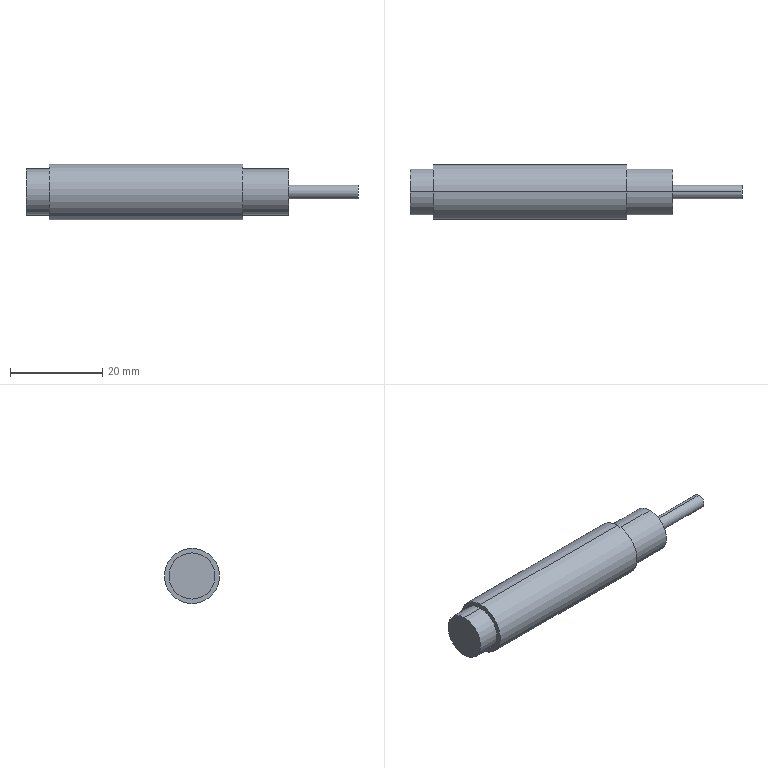Part | STEP file | PN_0014_default | 1 solid | 13 faces | box 72 x 12 x 12 mm | volume 6034 mm3 | cylinder 8 | plane 5 | commonest cylinder face diameters 10 x4 3 x2 12 x2
STEP:
#1=CARTESIAN_POINT('',(0.,0.,0.));
#2=DIRECTION('',(0.,0.,1.));
#3=DIRECTION('',(1.,0.,0.));
#4=AXIS2_PLACEMENT_3D('',#1,#2,#3);
#5=CARTESIAN_POINT('',(72.,0.,-1.5));
#6=VERTEX_POINT('',#5);
#7=CARTESIAN_POINT('',(72.,0.,1.5));
#8=VERTEX_POINT('',#7);
#9=CARTESIAN_POINT('',(72.,0.,0.));
#10=DIRECTION('',(1.,0.,0.));
#11=DIRECTION('',(0.,0.,-1.));
#12=AXIS2_PLACEMENT_3D('',#9,#10,#11);
#13=CIRCLE('',#12,1.5);
#14=CARTESIAN_POINT('',(72.,0.,0.));
#15=DIRECTION('',(-1.,0.,0.));
#16=DIRECTION('',(0.,0.,1.));
#17=AXIS2_PLACEMENT_3D('',#14,#15,#16);
#18=CYLINDRICAL_SURFACE('',#17,1.5);
#19=CARTESIAN_POINT('',(3.142,0.));
#20=DIRECTION('',(-1.,0.));
#21=VECTOR('',#20,1.);
#22=LINE('',#19,#21);
#23=(GEOMETRIC_REPRESENTATION_CONTEXT(2)PARAMETRIC_REPRESENTATION_CONTEXT()REPRESENTATION_CONTEXT('',''));
#24=DEFINITIONAL_REPRESENTATION('',(#22),#23);
#25=PCURVE('',#18,#24);
#26=CARTESIAN_POINT('',(72.,0.,0.));
#27=DIRECTION('',(1.,0.,0.));
#28=DIRECTION('',(0.,0.,-1.));
#29=AXIS2_PLACEMENT_3D('',#26,#27,#28);
#30=PLANE('',#29);
#31=CARTESIAN_POINT('',(0.,0.));
#32=DIRECTION('',(1.,0.));
#33=AXIS2_PLACEMENT_2D('',#31,#32);
#34=CIRCLE('',#33,1.5);
#35=(GEOMETRIC_REPRESENTATION_CONTEXT(2)PARAMETRIC_REPRESENTATION_CONTEXT()REPRESENTATION_CONTEXT('',''));
#36=DEFINITIONAL_REPRESENTATION('',(#34),#35);
#37=PCURVE('',#30,#36);
#38=SURFACE_CURVE('',#13,(#25,#37),.PCURVE_S1.);
#39=EDGE_CURVE('',#6,#8,#38,.T.);
#40=ORIENTED_EDGE('',*,*,#39,.F.);
#41=CARTESIAN_POINT('',(57.,0.,-1.5));
#42=VERTEX_POINT('',#41);
#43=CARTESIAN_POINT('',(72.,0.,-1.5));
#44=DIRECTION('',(-1.,0.,0.));
#45=VECTOR('',#44,1.);
#46=LINE('',#43,#45);
#47=CARTESIAN_POINT('',(3.142,0.));
#48=DIRECTION('',(0.,1.));
#49=VECTOR('',#48,1.);
#50=LINE('',#47,#49);
#51=(GEOMETRIC_REPRESENTATION_CONTEXT(2)PARAMETRIC_REPRESENTATION_CONTEXT()REPRESENTATION_CONTEXT('',''));
#52=DEFINITIONAL_REPRESENTATION('',(#50),#51);
#53=PCURVE('',#18,#52);
#54=CARTESIAN_POINT('',(72.,0.,0.));
#55=DIRECTION('',(-1.,0.,0.));
#56=DIRECTION('',(0.,0.,1.));
#57=AXIS2_PLACEMENT_3D('',#54,#55,#56);
#58=CYLINDRICAL_SURFACE('',#57,1.5);
#59=CARTESIAN_POINT('',(3.142,0.));
#60=DIRECTION('',(0.,1.));
#61=VECTOR('',#60,1.);
#62=LINE('',#59,#61);
#63=(GEOMETRIC_REPRESENTATION_CONTEXT(2)PARAMETRIC_REPRESENTATION_CONTEXT()REPRESENTATION_CONTEXT('',''));
#64=DEFINITIONAL_REPRESENTATION('',(#62),#63);
#65=PCURVE('',#58,#64);
#66=SURFACE_CURVE('',#46,(#53,#65),.PCURVE_S1.);
#67=EDGE_CURVE('',#6,#42,#66,.T.);
#68=ORIENTED_EDGE('',*,*,#67,.T.);
#69=CARTESIAN_POINT('',(57.,0.,1.5));
#70=VERTEX_POINT('',#69);
#71=CARTESIAN_POINT('',(57.,0.,0.));
#72=DIRECTION('',(1.,0.,0.));
#73=DIRECTION('',(0.,0.,1.));
#74=AXIS2_PLACEMENT_3D('',#71,#72,#73);
#75=CIRCLE('',#74,1.5);
#76=CARTESIAN_POINT('',(6.283,15.));
#77=DIRECTION('',(-1.,0.));
#78=VECTOR('',#77,1.);
#79=LINE('',#76,#78);
#80=(GEOMETRIC_REPRESENTATION_CONTEXT(2)PARAMETRIC_REPRESENTATION_CONTEXT()REPRESENTATION_CONTEXT('',''));
#81=DEFINITIONAL_REPRESENTATION('',(#79),#80);
#82=PCURVE('',#18,#81);
#83=CARTESIAN_POINT('',(57.,5.,0.));
#84=DIRECTION('',(-1.,0.,0.));
#85=DIRECTION('',(0.,0.,1.));
#86=AXIS2_PLACEMENT_3D('',#83,#84,#85);
#87=PLANE('',#86);
#88=CARTESIAN_POINT('',(1.5,-5.));
#89=CARTESIAN_POINT('',(1.5,-7.598));
#90=CARTESIAN_POINT('',(-0.75,-6.299));
#91=CARTESIAN_POINT('',(-3.,-5.));
#92=CARTESIAN_POINT('',(-0.75,-3.701));
#93=CARTESIAN_POINT('',(1.5,-2.402));
#94=CARTESIAN_POINT('',(1.5,-5.));
#95=(BOUNDED_CURVE()B_SPLINE_CURVE(2,(#88,#89,#90,#91,#92,#93,#94),.UNSPECIFIED.,.T.,.F.)B_SPLINE_CURVE_WITH_KNOTS((1,2,2,2,2,1),(-2.094,0.,2.094,4.189,6.283,8.378),.UNSPECIFIED.)CURVE()GEOMETRIC_REPRESENTATION_ITEM()RATIONAL_B_SPLINE_CURVE((1.,0.5,1.,0.5,1.,0.5,1.))REPRESENTATION_ITEM(''));
#96=(GEOMETRIC_REPRESENTATION_CONTEXT(2)PARAMETRIC_REPRESENTATION_CONTEXT()REPRESENTATION_CONTEXT('',''));
#97=DEFINITIONAL_REPRESENTATION('',(#95),#96);
#98=PCURVE('',#87,#97);
#99=SURFACE_CURVE('',#75,(#82,#98),.PCURVE_S1.);
#100=EDGE_CURVE('',#42,#70,#99,.T.);
#101=ORIENTED_EDGE('',*,*,#100,.T.);
#102=CARTESIAN_POINT('',(72.,0.,1.5));
#103=DIRECTION('',(-1.,0.,0.));
#104=VECTOR('',#103,1.);
#105=LINE('',#102,#104);
#106=CARTESIAN_POINT('',(0.,0.));
#107=DIRECTION('',(0.,1.));
#108=VECTOR('',#107,1.);
#109=LINE('',#106,#108);
#110=(GEOMETRIC_REPRESENTATION_CONTEXT(2)PARAMETRIC_REPRESENTATION_CONTEXT()REPRESENTATION_CONTEXT('',''));
#111=DEFINITIONAL_REPRESENTATION('',(#109),#110);
#112=PCURVE('',#18,#111);
#113=CARTESIAN_POINT('',(6.283,0.));
#114=DIRECTION('',(0.,1.));
#115=VECTOR('',#114,1.);
#116=LINE('',#113,#115);
#117=(GEOMETRIC_REPRESENTATION_CONTEXT(2)PARAMETRIC_REPRESENTATION_CONTEXT()REPRESENTATION_CONTEXT('',''));
#118=DEFINITIONAL_REPRESENTATION('',(#116),#117);
#119=PCURVE('',#58,#118);
#120=SURFACE_CURVE('',#105,(#112,#119),.PCURVE_S1.);
#121=EDGE_CURVE('',#8,#70,#120,.T.);
#122=ORIENTED_EDGE('',*,*,#121,.F.);
#123=EDGE_LOOP('',(#40,#68,#101,#122));
#124=FACE_BOUND('',#123,.T.);
#125=ADVANCED_FACE('',(#124),#18,.T.);
#126=CARTESIAN_POINT('',(57.,0.,5.));
#127=VERTEX_POINT('',#126);
#128=CARTESIAN_POINT('',(57.,0.,-5.));
#129=VERTEX_POINT('',#128);
#130=CARTESIAN_POINT('',(57.,0.,0.));
#131=DIRECTION('',(-1.,0.,0.));
#132=DIRECTION('',(0.,0.,1.));
#133=AXIS2_PLACEMENT_3D('',#130,#131,#132);
#134=CIRCLE('',#133,5.);
#135=CARTESIAN_POINT('',(0.,0.,0.));
#136=DIRECTION('',(-1.,0.,0.));
#137=DIRECTION('',(0.,0.,1.));
#138=AXIS2_PLACEMENT_3D('',#135,#136,#137);
#139=CYLINDRICAL_SURFACE('',#138,5.);
#140=CARTESIAN_POINT('',(0.,-57.));
#141=DIRECTION('',(1.,0.));
#142=VECTOR('',#141,1.);
#143=LINE('',#140,#142);
#144=(GEOMETRIC_REPRESENTATION_CONTEXT(2)PARAMETRIC_REPRESENTATION_CONTEXT()REPRESENTATION_CONTEXT('',''));
#145=DEFINITIONAL_REPRESENTATION('',(#143),#144);
#146=PCURVE('',#139,#145);
#147=CARTESIAN_POINT('',(0.,-5.));
#148=DIRECTION('',(1.,0.));
#149=AXIS2_PLACEMENT_2D('',#147,#148);
#150=CIRCLE('',#149,5.);
#151=(GEOMETRIC_REPRESENTATION_CONTEXT(2)PARAMETRIC_REPRESENTATION_CONTEXT()REPRESENTATION_CONTEXT('',''));
#152=DEFINITIONAL_REPRESENTATION('',(#150),#151);
#153=PCURVE('',#87,#152);
#154=SURFACE_CURVE('',#134,(#146,#153),.PCURVE_S1.);
#155=EDGE_CURVE('',#127,#129,#154,.T.);
#156=ORIENTED_EDGE('',*,*,#155,.T.);
#157=CARTESIAN_POINT('',(47.,0.,-5.));
#158=VERTEX_POINT('',#157);
#159=CARTESIAN_POINT('',(0.,0.,-5.));
#160=DIRECTION('',(-1.,0.,0.));
#161=VECTOR('',#160,1.);
#162=LINE('',#159,#161);
#163=CARTESIAN_POINT('',(3.142,0.));
#164=DIRECTION('',(0.,1.));
#165=VECTOR('',#164,1.);
#166=LINE('',#163,#165);
#167=(GEOMETRIC_REPRESENTATION_CONTEXT(2)PARAMETRIC_REPRESENTATION_CONTEXT()REPRESENTATION_CONTEXT('',''));
#168=DEFINITIONAL_REPRESENTATION('',(#166),#167);
#169=PCURVE('',#139,#168);
#170=CARTESIAN_POINT('',(0.,0.,0.));
#171=DIRECTION('',(-1.,0.,0.));
#172=DIRECTION('',(0.,0.,1.));
#173=AXIS2_PLACEMENT_3D('',#170,#171,#172);
#174=CYLINDRICAL_SURFACE('',#173,5.);
#175=CARTESIAN_POINT('',(3.142,0.));
#176=DIRECTION('',(0.,1.));
#177=VECTOR('',#176,1.);
#178=LINE('',#175,#177);
#179=(GEOMETRIC_REPRESENTATION_CONTEXT(2)PARAMETRIC_REPRESENTATION_CONTEXT()REPRESENTATION_CONTEXT('',''));
#180=DEFINITIONAL_REPRESENTATION('',(#178),#179);
#181=PCURVE('',#174,#180);
#182=SURFACE_CURVE('',#162,(#169,#181),.PCURVE_S1.);
#183=EDGE_CURVE('',#129,#158,#182,.T.);
#184=ORIENTED_EDGE('',*,*,#183,.T.);
#185=CARTESIAN_POINT('',(47.,0.,5.));
#186=VERTEX_POINT('',#185);
#187=CARTESIAN_POINT('',(47.,0.,0.));
#188=DIRECTION('',(-1.,0.,0.));
#189=DIRECTION('',(0.,0.,1.));
#190=AXIS2_PLACEMENT_3D('',#187,#188,#189);
#191=CIRCLE('',#190,5.);
#192=CARTESIAN_POINT('',(0.,-47.));
#193=DIRECTION('',(1.,0.));
#194=VECTOR('',#193,1.);
#195=LINE('',#192,#194);
#196=(GEOMETRIC_REPRESENTATION_CONTEXT(2)PARAMETRIC_REPRESENTATION_CONTEXT()REPRESENTATION_CONTEXT('',''));
#197=DEFINITIONAL_REPRESENTATION('',(#195),#196);
#198=PCURVE('',#139,#197);
#199=CARTESIAN_POINT('',(47.,6.,0.));
#200=DIRECTION('',(-1.,0.,0.));
#201=DIRECTION('',(0.,0.,1.));
#202=AXIS2_PLACEMENT_3D('',#199,#200,#201);
#203=PLANE('',#202);
#204=CARTESIAN_POINT('',(0.,-6.));
#205=DIRECTION('',(1.,0.));
#206=AXIS2_PLACEMENT_2D('',#204,#205);
#207=CIRCLE('',#206,5.);
#208=(GEOMETRIC_REPRESENTATION_CONTEXT(2)PARAMETRIC_REPRESENTATION_CONTEXT()REPRESENTATION_CONTEXT('',''));
#209=DEFINITIONAL_REPRESENTATION('',(#207),#208);
#210=PCURVE('',#203,#209);
#211=SURFACE_CURVE('',#191,(#198,#210),.PCURVE_S1.);
#212=EDGE_CURVE('',#186,#158,#211,.T.);
#213=ORIENTED_EDGE('',*,*,#212,.F.);
#214=CARTESIAN_POINT('',(0.,0.,5.));
#215=DIRECTION('',(-1.,0.,0.));
#216=VECTOR('',#215,1.);
#217=LINE('',#214,#216);
#218=CARTESIAN_POINT('',(0.,0.));
#219=DIRECTION('',(0.,1.));
#220=VECTOR('',#219,1.);
#221=LINE('',#218,#220);
#222=(GEOMETRIC_REPRESENTATION_CONTEXT(2)PARAMETRIC_REPRESENTATION_CONTEXT()REPRESENTATION_CONTEXT('',''));
#223=DEFINITIONAL_REPRESENTATION('',(#221),#222);
#224=PCURVE('',#139,#223);
#225=CARTESIAN_POINT('',(6.283,0.));
#226=DIRECTION('',(0.,1.));
#227=VECTOR('',#226,1.);
#228=LINE('',#225,#227);
#229=(GEOMETRIC_REPRESENTATION_CONTEXT(2)PARAMETRIC_REPRESENTATION_CONTEXT()REPRESENTATION_CONTEXT('',''));
#230=DEFINITIONAL_REPRESENTATION('',(#228),#229);
#231=PCURVE('',#174,#230);
#232=SURFACE_CURVE('',#217,(#224,#231),.PCURVE_S1.);
#233=EDGE_CURVE('',#127,#186,#232,.T.);
#234=ORIENTED_EDGE('',*,*,#233,.F.);
#235=EDGE_LOOP('',(#156,#184,#213,#234));
#236=FACE_BOUND('',#235,.T.);
#237=ADVANCED_FACE('',(#236),#139,.T.);
#238=CARTESIAN_POINT('',(47.,0.,6.));
#239=VERTEX_POINT('',#238);
#240=CARTESIAN_POINT('',(47.,0.,-6.));
#241=VERTEX_POINT('',#240);
#242=CARTESIAN_POINT('',(47.,0.,0.));
#243=DIRECTION('',(-1.,0.,0.));
#244=DIRECTION('',(0.,0.,1.));
#245=AXIS2_PLACEMENT_3D('',#242,#243,#244);
#246=CIRCLE('',#245,6.);
#247=CARTESIAN_POINT('',(0.,0.,0.));
#248=DIRECTION('',(-1.,0.,0.));
#249=DIRECTION('',(0.,0.,1.));
#250=AXIS2_PLACEMENT_3D('',#247,#248,#249);
#251=CYLINDRICAL_SURFACE('',#250,6.);
#252=CARTESIAN_POINT('',(0.,-47.));
#253=DIRECTION('',(1.,0.));
#254=VECTOR('',#253,1.);
#255=LINE('',#252,#254);
#256=(GEOMETRIC_REPRESENTATION_CONTEXT(2)PARAMETRIC_REPRESENTATION_CONTEXT()REPRESENTATION_CONTEXT('',''));
#257=DEFINITIONAL_REPRESENTATION('',(#255),#256);
#258=PCURVE('',#251,#257);
#259=CARTESIAN_POINT('',(0.,-6.));
#260=DIRECTION('',(1.,0.));
#261=AXIS2_PLACEMENT_2D('',#259,#260);
#262=CIRCLE('',#261,6.);
#263=(GEOMETRIC_REPRESENTATION_CONTEXT(2)PARAMETRIC_REPRESENTATION_CONTEXT()REPRESENTATION_CONTEXT('',''));
#264=DEFINITIONAL_REPRESENTATION('',(#262),#263);
#265=PCURVE('',#203,#264);
#266=SURFACE_CURVE('',#246,(#258,#265),.PCURVE_S1.);
#267=EDGE_CURVE('',#239,#241,#266,.T.);
#268=ORIENTED_EDGE('',*,*,#267,.T.);
#269=CARTESIAN_POINT('',(5.,0.,-6.));
#270=VERTEX_POINT('',#269);
#271=CARTESIAN_POINT('',(0.,0.,-6.));
#272=DIRECTION('',(-1.,0.,0.));
#273=VECTOR('',#272,1.);
#274=LINE('',#271,#273);
#275=CARTESIAN_POINT('',(3.142,0.));
#276=DIRECTION('',(0.,1.));
#277=VECTOR('',#276,1.);
#278=LINE('',#275,#277);
#279=(GEOMETRIC_REPRESENTATION_CONTEXT(2)PARAMETRIC_REPRESENTATION_CONTEXT()REPRESENTATION_CONTEXT('',''));
#280=DEFINITIONAL_REPRESENTATION('',(#278),#279);
#281=PCURVE('',#251,#280);
#282=CARTESIAN_POINT('',(0.,0.,0.));
#283=DIRECTION('',(-1.,0.,0.));
#284=DIRECTION('',(0.,0.,1.));
#285=AXIS2_PLACEMENT_3D('',#282,#283,#284);
#286=CYLINDRICAL_SURFACE('',#285,6.);
#287=CARTESIAN_POINT('',(3.142,0.));
#288=DIRECTION('',(0.,1.));
#289=VECTOR('',#288,1.);
#290=LINE('',#287,#289);
#291=(GEOMETRIC_REPRESENTATION_CONTEXT(2)PARAMETRIC_REPRESENTATION_CONTEXT()REPRESENTATION_CONTEXT('',''));
#292=DEFINITIONAL_REPRESENTATION('',(#290),#291);
#293=PCURVE('',#286,#292);
#294=SURFACE_CURVE('',#274,(#281,#293),.PCURVE_S1.);
#295=EDGE_CURVE('',#241,#270,#294,.T.);
#296=ORIENTED_EDGE('',*,*,#295,.T.);
#297=CARTESIAN_POINT('',(5.,0.,6.));
#298=VERTEX_POINT('',#297);
#299=CARTESIAN_POINT('',(5.,0.,0.));
#300=DIRECTION('',(-1.,0.,0.));
#301=DIRECTION('',(0.,0.,1.));
#302=AXIS2_PLACEMENT_3D('',#299,#300,#301);
#303=CIRCLE('',#302,6.);
#304=CARTESIAN_POINT('',(0.,-5.));
#305=DIRECTION('',(1.,0.));
#306=VECTOR('',#305,1.);
#307=LINE('',#304,#306);
#308=(GEOMETRIC_REPRESENTATION_CONTEXT(2)PARAMETRIC_REPRESENTATION_CONTEXT()REPRESENTATION_CONTEXT('',''));
#309=DEFINITIONAL_REPRESENTATION('',(#307),#308);
#310=PCURVE('',#251,#309);
#311=CARTESIAN_POINT('',(5.,5.,0.));
#312=DIRECTION('',(1.,0.,0.));
#313=DIRECTION('',(0.,0.,-1.));
#314=AXIS2_PLACEMENT_3D('',#311,#312,#313);
#315=PLANE('',#314);
#316=CARTESIAN_POINT('',(-6.,-5.));
#317=CARTESIAN_POINT('',(-6.,5.392));
#318=CARTESIAN_POINT('',(3.,0.1962));
#319=CARTESIAN_POINT('',(12.,-5.));
#320=CARTESIAN_POINT('',(3.,-10.196));
#321=CARTESIAN_POINT('',(-6.,-15.392));
#322=CARTESIAN_POINT('',(-6.,-5.));
#323=(BOUNDED_CURVE()B_SPLINE_CURVE(2,(#316,#317,#318,#319,#320,#321,#322),.UNSPECIFIED.,.T.,.F.)B_SPLINE_CURVE_WITH_KNOTS((1,2,2,2,2,1),(-2.094,0.,2.094,4.189,6.283,8.378),.UNSPECIFIED.)CURVE()GEOMETRIC_REPRESENTATION_ITEM()RATIONAL_B_SPLINE_CURVE((1.,0.5,1.,0.5,1.,0.5,1.))REPRESENTATION_ITEM(''));
#324=(GEOMETRIC_REPRESENTATION_CONTEXT(2)PARAMETRIC_REPRESENTATION_CONTEXT()REPRESENTATION_CONTEXT('',''));
#325=DEFINITIONAL_REPRESENTATION('',(#323),#324);
#326=PCURVE('',#315,#325);
#327=SURFACE_CURVE('',#303,(#310,#326),.PCURVE_S1.);
#328=EDGE_CURVE('',#298,#270,#327,.T.);
#329=ORIENTED_EDGE('',*,*,#328,.F.);
#330=CARTESIAN_POINT('',(0.,0.,6.));
#331=DIRECTION('',(-1.,0.,0.));
#332=VECTOR('',#331,1.);
#333=LINE('',#330,#332);
#334=CARTESIAN_POINT('',(0.,0.));
#335=DIRECTION('',(0.,1.));
#336=VECTOR('',#335,1.);
#337=LINE('',#334,#336);
#338=(GEOMETRIC_REPRESENTATION_CONTEXT(2)PARAMETRIC_REPRESENTATION_CONTEXT()REPRESENTATION_CONTEXT('',''));
#339=DEFINITIONAL_REPRESENTATION('',(#337),#338);
#340=PCURVE('',#251,#339);
#341=CARTESIAN_POINT('',(6.283,0.));
#342=DIRECTION('',(0.,1.));
#343=VECTOR('',#342,1.);
#344=LINE('',#341,#343);
#345=(GEOMETRIC_REPRESENTATION_CONTEXT(2)PARAMETRIC_REPRESENTATION_CONTEXT()REPRESENTATION_CONTEXT('',''));
#346=DEFINITIONAL_REPRESENTATION('',(#344),#345);
#347=PCURVE('',#286,#346);
#348=SURFACE_CURVE('',#333,(#340,#347),.PCURVE_S1.);
#349=EDGE_CURVE('',#239,#298,#348,.T.);
#350=ORIENTED_EDGE('',*,*,#349,.F.);
#351=EDGE_LOOP('',(#268,#296,#329,#350));
#352=FACE_BOUND('',#351,.T.);
#353=ADVANCED_FACE('',(#352),#251,.T.);
#354=CARTESIAN_POINT('',(5.,0.,5.));
#355=VERTEX_POINT('',#354);
#356=CARTESIAN_POINT('',(5.,0.,-5.));
#357=VERTEX_POINT('',#356);
#358=CARTESIAN_POINT('',(5.,0.,0.));
#359=DIRECTION('',(-1.,0.,0.));
#360=DIRECTION('',(0.,0.,1.));
#361=AXIS2_PLACEMENT_3D('',#358,#359,#360);
#362=CIRCLE('',#361,5.);
#363=CARTESIAN_POINT('',(0.,0.,0.));
#364=DIRECTION('',(-1.,0.,0.));
#365=DIRECTION('',(0.,0.,1.));
#366=AXIS2_PLACEMENT_3D('',#363,#364,#365);
#367=CYLINDRICAL_SURFACE('',#366,5.);
#368=CARTESIAN_POINT('',(0.,-5.));
#369=DIRECTION('',(1.,0.));
#370=VECTOR('',#369,1.);
#371=LINE('',#368,#370);
#372=(GEOMETRIC_REPRESENTATION_CONTEXT(2)PARAMETRIC_REPRESENTATION_CONTEXT()REPRESENTATION_CONTEXT('',''));
#373=DEFINITIONAL_REPRESENTATION('',(#371),#372);
#374=PCURVE('',#367,#373);
#375=CARTESIAN_POINT('',(-5.,-5.));
#376=CARTESIAN_POINT('',(-5.,3.66));
#377=CARTESIAN_POINT('',(2.5,-0.6699));
#378=CARTESIAN_POINT('',(10.,-5.));
#379=CARTESIAN_POINT('',(2.5,-9.33));
#380=CARTESIAN_POINT('',(-5.,-13.66));
#381=CARTESIAN_POINT('',(-5.,-5.));
#382=(BOUNDED_CURVE()B_SPLINE_CURVE(2,(#375,#376,#377,#378,#379,#380,#381),.UNSPECIFIED.,.T.,.F.)B_SPLINE_CURVE_WITH_KNOTS((1,2,2,2,2,1),(-2.094,0.,2.094,4.189,6.283,8.378),.UNSPECIFIED.)CURVE()GEOMETRIC_REPRESENTATION_ITEM()RATIONAL_B_SPLINE_CURVE((1.,0.5,1.,0.5,1.,0.5,1.))REPRESENTATION_ITEM(''));
#383=(GEOMETRIC_REPRESENTATION_CONTEXT(2)PARAMETRIC_REPRESENTATION_CONTEXT()REPRESENTATION_CONTEXT('',''));
#384=DEFINITIONAL_REPRESENTATION('',(#382),#383);
#385=PCURVE('',#315,#384);
#386=SURFACE_CURVE('',#362,(#374,#385),.PCURVE_S1.);
#387=EDGE_CURVE('',#355,#357,#386,.T.);
#388=ORIENTED_EDGE('',*,*,#387,.T.);
#389=CARTESIAN_POINT('',(0.,0.,-5.));
#390=VERTEX_POINT('',#389);
#391=CARTESIAN_POINT('',(0.,0.,-5.));
#392=DIRECTION('',(-1.,0.,0.));
#393=VECTOR('',#392,1.);
#394=LINE('',#391,#393);
#395=CARTESIAN_POINT('',(3.142,0.));
#396=DIRECTION('',(0.,1.));
#397=VECTOR('',#396,1.);
#398=LINE('',#395,#397);
#399=(GEOMETRIC_REPRESENTATION_CONTEXT(2)PARAMETRIC_REPRESENTATION_CONTEXT()REPRESENTATION_CONTEXT('',''));
#400=DEFINITIONAL_REPRESENTATION('',(#398),#399);
#401=PCURVE('',#367,#400);
#402=CARTESIAN_POINT('',(0.,0.,0.));
#403=DIRECTION('',(-1.,0.,0.));
#404=DIRECTION('',(0.,0.,1.));
#405=AXIS2_PLACEMENT_3D('',#402,#403,#404);
#406=CYLINDRICAL_SURFACE('',#405,5.);
#407=CARTESIAN_POINT('',(3.142,0.));
#408=DIRECTION('',(0.,1.));
#409=VECTOR('',#408,1.);
#410=LINE('',#407,#409);
#411=(GEOMETRIC_REPRESENTATION_CONTEXT(2)PARAMETRIC_REPRESENTATION_CONTEXT()REPRESENTATION_CONTEXT('',''));
#412=DEFINITIONAL_REPRESENTATION('',(#410),#411);
#413=PCURVE('',#406,#412);
#414=SURFACE_CURVE('',#394,(#401,#413),.PCURVE_S1.);
#415=EDGE_CURVE('',#357,#390,#414,.T.);
#416=ORIENTED_EDGE('',*,*,#415,.T.);
#417=CARTESIAN_POINT('',(0.,0.,5.));
#418=VERTEX_POINT('',#417);
#419=CARTESIAN_POINT('',(0.,0.,0.));
#420=DIRECTION('',(-1.,0.,0.));
#421=DIRECTION('',(0.,0.,1.));
#422=AXIS2_PLACEMENT_3D('',#419,#420,#421);
#423=CIRCLE('',#422,5.);
#424=CARTESIAN_POINT('',(0.,0.));
#425=DIRECTION('',(1.,0.));
#426=VECTOR('',#425,1.);
#427=LINE('',#424,#426);
#428=(GEOMETRIC_REPRESENTATION_CONTEXT(2)PARAMETRIC_REPRESENTATION_CONTEXT()REPRESENTATION_CONTEXT('',''));
#429=DEFINITIONAL_REPRESENTATION('',(#427),#428);
#430=PCURVE('',#367,#429);
#431=CARTESIAN_POINT('',(0.,0.,0.));
#432=DIRECTION('',(1.,0.,0.));
#433=DIRECTION('',(0.,0.,-1.));
#434=AXIS2_PLACEMENT_3D('',#431,#432,#433);
#435=PLANE('',#434);
#436=CARTESIAN_POINT('',(-5.,0.));
#437=CARTESIAN_POINT('',(-5.,8.66));
#438=CARTESIAN_POINT('',(2.5,4.33));
#439=CARTESIAN_POINT('',(10.,0.));
#440=CARTESIAN_POINT('',(2.5,-4.33));
#441=CARTESIAN_POINT('',(-5.,-8.66));
#442=CARTESIAN_POINT('',(-5.,0.));
#443=(BOUNDED_CURVE()B_SPLINE_CURVE(2,(#436,#437,#438,#439,#440,#441,#442),.UNSPECIFIED.,.T.,.F.)B_SPLINE_CURVE_WITH_KNOTS((1,2,2,2,2,1),(-2.094,0.,2.094,4.189,6.283,8.378),.UNSPECIFIED.)CURVE()GEOMETRIC_REPRESENTATION_ITEM()RATIONAL_B_SPLINE_CURVE((1.,0.5,1.,0.5,1.,0.5,1.))REPRESENTATION_ITEM(''));
#444=(GEOMETRIC_REPRESENTATION_CONTEXT(2)PARAMETRIC_REPRESENTATION_CONTEXT()REPRESENTATION_CONTEXT('',''));
#445=DEFINITIONAL_REPRESENTATION('',(#443),#444);
#446=PCURVE('',#435,#445);
#447=SURFACE_CURVE('',#423,(#430,#446),.PCURVE_S1.);
#448=EDGE_CURVE('',#418,#390,#447,.T.);
#449=ORIENTED_EDGE('',*,*,#448,.F.);
#450=CARTESIAN_POINT('',(0.,0.,5.));
#451=DIRECTION('',(-1.,0.,0.));
#452=VECTOR('',#451,1.);
#453=LINE('',#450,#452);
#454=CARTESIAN_POINT('',(0.,0.));
#455=DIRECTION('',(0.,1.));
#456=VECTOR('',#455,1.);
#457=LINE('',#454,#456);
#458=(GEOMETRIC_REPRESENTATION_CONTEXT(2)PARAMETRIC_REPRESENTATION_CONTEXT()REPRESENTATION_CONTEXT('',''));
#459=DEFINITIONAL_REPRESENTATION('',(#457),#458);
#460=PCURVE('',#367,#459);
#461=CARTESIAN_POINT('',(6.283,0.));
#462=DIRECTION('',(0.,1.));
#463=VECTOR('',#462,1.);
#464=LINE('',#461,#463);
#465=(GEOMETRIC_REPRESENTATION_CONTEXT(2)PARAMETRIC_REPRESENTATION_CONTEXT()REPRESENTATION_CONTEXT('',''));
#466=DEFINITIONAL_REPRESENTATION('',(#464),#465);
#467=PCURVE('',#406,#466);
#468=SURFACE_CURVE('',#453,(#460,#467),.PCURVE_S1.);
#469=EDGE_CURVE('',#355,#418,#468,.T.);
#470=ORIENTED_EDGE('',*,*,#469,.F.);
#471=EDGE_LOOP('',(#388,#416,#449,#470));
#472=FACE_BOUND('',#471,.T.);
#473=ADVANCED_FACE('',(#472),#367,.T.);
#474=ORIENTED_EDGE('',*,*,#155,.F.);
#475=CARTESIAN_POINT('',(57.,0.,0.));
#476=DIRECTION('',(-1.,0.,0.));
#477=DIRECTION('',(0.,0.,1.));
#478=AXIS2_PLACEMENT_3D('',#475,#476,#477);
#479=CIRCLE('',#478,5.);
#480=CARTESIAN_POINT('',(0.,-5.));
#481=DIRECTION('',(1.,0.));
#482=AXIS2_PLACEMENT_2D('',#480,#481);
#483=CIRCLE('',#482,5.);
#484=(GEOMETRIC_REPRESENTATION_CONTEXT(2)PARAMETRIC_REPRESENTATION_CONTEXT()REPRESENTATION_CONTEXT('',''));
#485=DEFINITIONAL_REPRESENTATION('',(#483),#484);
#486=PCURVE('',#87,#485);
#487=CARTESIAN_POINT('',(0.,-57.));
#488=DIRECTION('',(1.,0.));
#489=VECTOR('',#488,1.);
#490=LINE('',#487,#489);
#491=(GEOMETRIC_REPRESENTATION_CONTEXT(2)PARAMETRIC_REPRESENTATION_CONTEXT()REPRESENTATION_CONTEXT('',''));
#492=DEFINITIONAL_REPRESENTATION('',(#490),#491);
#493=PCURVE('',#174,#492);
#494=SURFACE_CURVE('',#479,(#486,#493),.PCURVE_S1.);
#495=EDGE_CURVE('',#129,#127,#494,.T.);
#496=ORIENTED_EDGE('',*,*,#495,.F.);
#497=EDGE_LOOP('',(#474,#496));
#498=FACE_BOUND('',#497,.T.);
#499=CARTESIAN_POINT('',(57.,0.,0.));
#500=DIRECTION('',(1.,0.,0.));
#501=DIRECTION('',(0.,0.,1.));
#502=AXIS2_PLACEMENT_3D('',#499,#500,#501);
#503=CIRCLE('',#502,1.5);
#504=CARTESIAN_POINT('',(1.5,-5.));
#505=CARTESIAN_POINT('',(1.5,-7.598));
#506=CARTESIAN_POINT('',(-0.75,-6.299));
#507=CARTESIAN_POINT('',(-3.,-5.));
#508=CARTESIAN_POINT('',(-0.75,-3.701));
#509=CARTESIAN_POINT('',(1.5,-2.402));
#510=CARTESIAN_POINT('',(1.5,-5.));
#511=(BOUNDED_CURVE()B_SPLINE_CURVE(2,(#504,#505,#506,#507,#508,#509,#510),.UNSPECIFIED.,.T.,.F.)B_SPLINE_CURVE_WITH_KNOTS((1,2,2,2,2,1),(-2.094,0.,2.094,4.189,6.283,8.378),.UNSPECIFIED.)CURVE()GEOMETRIC_REPRESENTATION_ITEM()RATIONAL_B_SPLINE_CURVE((1.,0.5,1.,0.5,1.,0.5,1.))REPRESENTATION_ITEM(''));
#512=(GEOMETRIC_REPRESENTATION_CONTEXT(2)PARAMETRIC_REPRESENTATION_CONTEXT()REPRESENTATION_CONTEXT('',''));
#513=DEFINITIONAL_REPRESENTATION('',(#511),#512);
#514=PCURVE('',#87,#513);
#515=CARTESIAN_POINT('',(6.283,15.));
#516=DIRECTION('',(-1.,0.));
#517=VECTOR('',#516,1.);
#518=LINE('',#515,#517);
#519=(GEOMETRIC_REPRESENTATION_CONTEXT(2)PARAMETRIC_REPRESENTATION_CONTEXT()REPRESENTATION_CONTEXT('',''));
#520=DEFINITIONAL_REPRESENTATION('',(#518),#519);
#521=PCURVE('',#58,#520);
#522=SURFACE_CURVE('',#503,(#514,#521),.PCURVE_S1.);
#523=EDGE_CURVE('',#70,#42,#522,.T.);
#524=ORIENTED_EDGE('',*,*,#523,.F.);
#525=ORIENTED_EDGE('',*,*,#100,.F.);
#526=EDGE_LOOP('',(#524,#525));
#527=FACE_BOUND('',#526,.T.);
#528=ADVANCED_FACE('',(#498,#527),#87,.F.);
#529=ORIENTED_EDGE('',*,*,#448,.T.);
#530=CARTESIAN_POINT('',(0.,0.,0.));
#531=DIRECTION('',(-1.,0.,0.));
#532=DIRECTION('',(0.,0.,1.));
#533=AXIS2_PLACEMENT_3D('',#530,#531,#532);
#534=CIRCLE('',#533,5.);
#535=CARTESIAN_POINT('',(-5.,0.));
#536=CARTESIAN_POINT('',(-5.,8.66));
#537=CARTESIAN_POINT('',(2.5,4.33));
#538=CARTESIAN_POINT('',(10.,0.));
#539=CARTESIAN_POINT('',(2.5,-4.33));
#540=CARTESIAN_POINT('',(-5.,-8.66));
#541=CARTESIAN_POINT('',(-5.,0.));
#542=(BOUNDED_CURVE()B_SPLINE_CURVE(2,(#535,#536,#537,#538,#539,#540,#541),.UNSPECIFIED.,.T.,.F.)B_SPLINE_CURVE_WITH_KNOTS((1,2,2,2,2,1),(-2.094,0.,2.094,4.189,6.283,8.378),.UNSPECIFIED.)CURVE()GEOMETRIC_REPRESENTATION_ITEM()RATIONAL_B_SPLINE_CURVE((1.,0.5,1.,0.5,1.,0.5,1.))REPRESENTATION_ITEM(''));
#543=(GEOMETRIC_REPRESENTATION_CONTEXT(2)PARAMETRIC_REPRESENTATION_CONTEXT()REPRESENTATION_CONTEXT('',''));
#544=DEFINITIONAL_REPRESENTATION('',(#542),#543);
#545=PCURVE('',#435,#544);
#546=CARTESIAN_POINT('',(0.,0.));
#547=DIRECTION('',(1.,0.));
#548=VECTOR('',#547,1.);
#549=LINE('',#546,#548);
#550=(GEOMETRIC_REPRESENTATION_CONTEXT(2)PARAMETRIC_REPRESENTATION_CONTEXT()REPRESENTATION_CONTEXT('',''));
#551=DEFINITIONAL_REPRESENTATION('',(#549),#550);
#552=PCURVE('',#406,#551);
#553=SURFACE_CURVE('',#534,(#545,#552),.PCURVE_S1.);
#554=EDGE_CURVE('',#390,#418,#553,.T.);
#555=ORIENTED_EDGE('',*,*,#554,.T.);
#556=EDGE_LOOP('',(#529,#555));
#557=FACE_BOUND('',#556,.T.);
#558=ADVANCED_FACE('',(#557),#435,.F.);
#559=ORIENTED_EDGE('',*,*,#415,.F.);
#560=CARTESIAN_POINT('',(5.,0.,0.));
#561=DIRECTION('',(-1.,0.,0.));
#562=DIRECTION('',(0.,0.,1.));
#563=AXIS2_PLACEMENT_3D('',#560,#561,#562);
#564=CIRCLE('',#563,5.);
#565=CARTESIAN_POINT('',(0.,-5.));
#566=DIRECTION('',(1.,0.));
#567=VECTOR('',#566,1.);
#568=LINE('',#565,#567);
#569=(GEOMETRIC_REPRESENTATION_CONTEXT(2)PARAMETRIC_REPRESENTATION_CONTEXT()REPRESENTATION_CONTEXT('',''));
#570=DEFINITIONAL_REPRESENTATION('',(#568),#569);
#571=PCURVE('',#406,#570);
#572=CARTESIAN_POINT('',(-5.,-5.));
#573=CARTESIAN_POINT('',(-5.,3.66));
#574=CARTESIAN_POINT('',(2.5,-0.6699));
#575=CARTESIAN_POINT('',(10.,-5.));
#576=CARTESIAN_POINT('',(2.5,-9.33));
#577=CARTESIAN_POINT('',(-5.,-13.66));
#578=CARTESIAN_POINT('',(-5.,-5.));
#579=(BOUNDED_CURVE()B_SPLINE_CURVE(2,(#572,#573,#574,#575,#576,#577,#578),.UNSPECIFIED.,.T.,.F.)B_SPLINE_CURVE_WITH_KNOTS((1,2,2,2,2,1),(-2.094,0.,2.094,4.189,6.283,8.378),.UNSPECIFIED.)CURVE()GEOMETRIC_REPRESENTATION_ITEM()RATIONAL_B_SPLINE_CURVE((1.,0.5,1.,0.5,1.,0.5,1.))REPRESENTATION_ITEM(''));
#580=(GEOMETRIC_REPRESENTATION_CONTEXT(2)PARAMETRIC_REPRESENTATION_CONTEXT()REPRESENTATION_CONTEXT('',''));
#581=DEFINITIONAL_REPRESENTATION('',(#579),#580);
#582=PCURVE('',#315,#581);
#583=SURFACE_CURVE('',#564,(#571,#582),.PCURVE_S1.);
#584=EDGE_CURVE('',#357,#355,#583,.T.);
#585=ORIENTED_EDGE('',*,*,#584,.T.);
#586=ORIENTED_EDGE('',*,*,#469,.T.);
#587=ORIENTED_EDGE('',*,*,#554,.F.);
#588=EDGE_LOOP('',(#559,#585,#586,#587));
#589=FACE_BOUND('',#588,.T.);
#590=ADVANCED_FACE('',(#589),#406,.T.);
#591=ORIENTED_EDGE('',*,*,#387,.F.);
#592=ORIENTED_EDGE('',*,*,#584,.F.);
#593=EDGE_LOOP('',(#591,#592));
#594=FACE_BOUND('',#593,.T.);
#595=ORIENTED_EDGE('',*,*,#328,.T.);
#596=CARTESIAN_POINT('',(5.,0.,0.));
#597=DIRECTION('',(-1.,0.,0.));
#598=DIRECTION('',(0.,0.,1.));
#599=AXIS2_PLACEMENT_3D('',#596,#597,#598);
#600=CIRCLE('',#599,6.);
#601=CARTESIAN_POINT('',(-6.,-5.));
#602=CARTESIAN_POINT('',(-6.,5.392));
#603=CARTESIAN_POINT('',(3.,0.1962));
#604=CARTESIAN_POINT('',(12.,-5.));
#605=CARTESIAN_POINT('',(3.,-10.196));
#606=CARTESIAN_POINT('',(-6.,-15.392));
#607=CARTESIAN_POINT('',(-6.,-5.));
#608=(BOUNDED_CURVE()B_SPLINE_CURVE(2,(#601,#602,#603,#604,#605,#606,#607),.UNSPECIFIED.,.T.,.F.)B_SPLINE_CURVE_WITH_KNOTS((1,2,2,2,2,1),(-2.094,0.,2.094,4.189,6.283,8.378),.UNSPECIFIED.)CURVE()GEOMETRIC_REPRESENTATION_ITEM()RATIONAL_B_SPLINE_CURVE((1.,0.5,1.,0.5,1.,0.5,1.))REPRESENTATION_ITEM(''));
#609=(GEOMETRIC_REPRESENTATION_CONTEXT(2)PARAMETRIC_REPRESENTATION_CONTEXT()REPRESENTATION_CONTEXT('',''));
#610=DEFINITIONAL_REPRESENTATION('',(#608),#609);
#611=PCURVE('',#315,#610);
#612=CARTESIAN_POINT('',(0.,-5.));
#613=DIRECTION('',(1.,0.));
#614=VECTOR('',#613,1.);
#615=LINE('',#612,#614);
#616=(GEOMETRIC_REPRESENTATION_CONTEXT(2)PARAMETRIC_REPRESENTATION_CONTEXT()REPRESENTATION_CONTEXT('',''));
#617=DEFINITIONAL_REPRESENTATION('',(#615),#616);
#618=PCURVE('',#286,#617);
#619=SURFACE_CURVE('',#600,(#611,#618),.PCURVE_S1.);
#620=EDGE_CURVE('',#270,#298,#619,.T.);
#621=ORIENTED_EDGE('',*,*,#620,.T.);
#622=EDGE_LOOP('',(#595,#621));
#623=FACE_BOUND('',#622,.T.);
#624=ADVANCED_FACE('',(#594,#623),#315,.F.);
#625=ORIENTED_EDGE('',*,*,#295,.F.);
#626=CARTESIAN_POINT('',(47.,0.,0.));
#627=DIRECTION('',(-1.,0.,0.));
#628=DIRECTION('',(0.,0.,1.));
#629=AXIS2_PLACEMENT_3D('',#626,#627,#628);
#630=CIRCLE('',#629,6.);
#631=CARTESIAN_POINT('',(0.,-47.));
#632=DIRECTION('',(1.,0.));
#633=VECTOR('',#632,1.);
#634=LINE('',#631,#633);
#635=(GEOMETRIC_REPRESENTATION_CONTEXT(2)PARAMETRIC_REPRESENTATION_CONTEXT()REPRESENTATION_CONTEXT('',''));
#636=DEFINITIONAL_REPRESENTATION('',(#634),#635);
#637=PCURVE('',#286,#636);
#638=CARTESIAN_POINT('',(0.,-6.));
#639=DIRECTION('',(1.,0.));
#640=AXIS2_PLACEMENT_2D('',#638,#639);
#641=CIRCLE('',#640,6.);
#642=(GEOMETRIC_REPRESENTATION_CONTEXT(2)PARAMETRIC_REPRESENTATION_CONTEXT()REPRESENTATION_CONTEXT('',''));
#643=DEFINITIONAL_REPRESENTATION('',(#641),#642);
#644=PCURVE('',#203,#643);
#645=SURFACE_CURVE('',#630,(#637,#644),.PCURVE_S1.);
#646=EDGE_CURVE('',#241,#239,#645,.T.);
#647=ORIENTED_EDGE('',*,*,#646,.T.);
#648=ORIENTED_EDGE('',*,*,#349,.T.);
#649=ORIENTED_EDGE('',*,*,#620,.F.);
#650=EDGE_LOOP('',(#625,#647,#648,#649));
#651=FACE_BOUND('',#650,.T.);
#652=ADVANCED_FACE('',(#651),#286,.T.);
#653=ORIENTED_EDGE('',*,*,#267,.F.);
#654=ORIENTED_EDGE('',*,*,#646,.F.);
#655=EDGE_LOOP('',(#653,#654));
#656=FACE_BOUND('',#655,.T.);
#657=ORIENTED_EDGE('',*,*,#212,.T.);
#658=CARTESIAN_POINT('',(47.,0.,0.));
#659=DIRECTION('',(-1.,0.,0.));
#660=DIRECTION('',(0.,0.,1.));
#661=AXIS2_PLACEMENT_3D('',#658,#659,#660);
#662=CIRCLE('',#661,5.);
#663=CARTESIAN_POINT('',(0.,-6.));
#664=DIRECTION('',(1.,0.));
#665=AXIS2_PLACEMENT_2D('',#663,#664);
#666=CIRCLE('',#665,5.);
#667=(GEOMETRIC_REPRESENTATION_CONTEXT(2)PARAMETRIC_REPRESENTATION_CONTEXT()REPRESENTATION_CONTEXT('',''));
#668=DEFINITIONAL_REPRESENTATION('',(#666),#667);
#669=PCURVE('',#203,#668);
#670=CARTESIAN_POINT('',(0.,-47.));
#671=DIRECTION('',(1.,0.));
#672=VECTOR('',#671,1.);
#673=LINE('',#670,#672);
#674=(GEOMETRIC_REPRESENTATION_CONTEXT(2)PARAMETRIC_REPRESENTATION_CONTEXT()REPRESENTATION_CONTEXT('',''));
#675=DEFINITIONAL_REPRESENTATION('',(#673),#674);
#676=PCURVE('',#174,#675);
#677=SURFACE_CURVE('',#662,(#669,#676),.PCURVE_S1.);
#678=EDGE_CURVE('',#158,#186,#677,.T.);
#679=ORIENTED_EDGE('',*,*,#678,.T.);
#680=EDGE_LOOP('',(#657,#679));
#681=FACE_BOUND('',#680,.T.);
#682=ADVANCED_FACE('',(#656,#681),#203,.F.);
#683=ORIENTED_EDGE('',*,*,#183,.F.);
#684=ORIENTED_EDGE('',*,*,#495,.T.);
#685=ORIENTED_EDGE('',*,*,#233,.T.);
#686=ORIENTED_EDGE('',*,*,#678,.F.);
#687=EDGE_LOOP('',(#683,#684,#685,#686));
#688=FACE_BOUND('',#687,.T.);
#689=ADVANCED_FACE('',(#688),#174,.T.);
#690=ORIENTED_EDGE('',*,*,#67,.F.);
#691=CARTESIAN_POINT('',(72.,0.,0.));
#692=DIRECTION('',(1.,0.,0.));
#693=DIRECTION('',(0.,0.,-1.));
#694=AXIS2_PLACEMENT_3D('',#691,#692,#693);
#695=CIRCLE('',#694,1.5);
#696=CARTESIAN_POINT('',(9.425,0.));
#697=DIRECTION('',(-1.,0.));
#698=VECTOR('',#697,1.);
#699=LINE('',#696,#698);
#700=(GEOMETRIC_REPRESENTATION_CONTEXT(2)PARAMETRIC_REPRESENTATION_CONTEXT()REPRESENTATION_CONTEXT('',''));
#701=DEFINITIONAL_REPRESENTATION('',(#699),#700);
#702=PCURVE('',#58,#701);
#703=CARTESIAN_POINT('',(0.,0.));
#704=DIRECTION('',(1.,0.));
#705=AXIS2_PLACEMENT_2D('',#703,#704);
#706=CIRCLE('',#705,1.5);
#707=(GEOMETRIC_REPRESENTATION_CONTEXT(2)PARAMETRIC_REPRESENTATION_CONTEXT()REPRESENTATION_CONTEXT('',''));
#708=DEFINITIONAL_REPRESENTATION('',(#706),#707);
#709=PCURVE('',#30,#708);
#710=SURFACE_CURVE('',#695,(#702,#709),.PCURVE_S1.);
#711=EDGE_CURVE('',#8,#6,#710,.T.);
#712=ORIENTED_EDGE('',*,*,#711,.F.);
#713=ORIENTED_EDGE('',*,*,#121,.T.);
#714=ORIENTED_EDGE('',*,*,#523,.T.);
#715=EDGE_LOOP('',(#690,#712,#713,#714));
#716=FACE_BOUND('',#715,.T.);
#717=ADVANCED_FACE('',(#716),#58,.T.);
#718=ORIENTED_EDGE('',*,*,#711,.T.);
#719=ORIENTED_EDGE('',*,*,#39,.T.);
#720=EDGE_LOOP('',(#718,#719));
#721=FACE_BOUND('',#720,.T.);
#722=ADVANCED_FACE('',(#721),#30,.T.);
#723=CLOSED_SHELL('',(#125,#237,#353,#473,#528,#558,#590,#624,#652,#682,#689,#717,#722));
#724=MANIFOLD_SOLID_BREP('',#723);
#725=(LENGTH_UNIT()NAMED_UNIT(*)SI_UNIT(.MILLI.,.METRE.));
#726=UNCERTAINTY_MEASURE_WITH_UNIT(LENGTH_MEASURE(0.0000001),#725,'','');
#727=(NAMED_UNIT(*)PLANE_ANGLE_UNIT()SI_UNIT($,.RADIAN.));
#728=(NAMED_UNIT(*)SI_UNIT($,.STERADIAN.)SOLID_ANGLE_UNIT());
#729=(GEOMETRIC_REPRESENTATION_CONTEXT(3)GLOBAL_UNCERTAINTY_ASSIGNED_CONTEXT((#726))GLOBAL_UNIT_ASSIGNED_CONTEXT((#725,#727,#728))REPRESENTATION_CONTEXT('',''));
#730=ADVANCED_BREP_SHAPE_REPRESENTATION('',(#4,#724),#729);